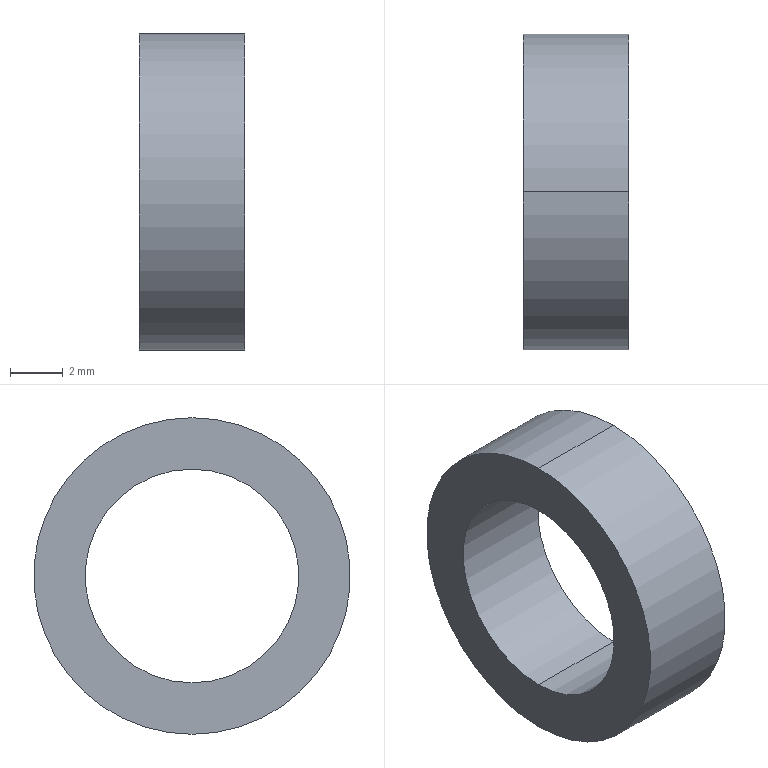Part | SolidWorks | features BaseBody 1 | 1 solid | 6 faces | box 4 x 12 x 12 mm | volume 246.269 mm3 | cylinder 4 | plane 2 | commonest cylinder face diameters 8.1 x2 12 x2
STEP:
#1=CARTESIAN_POINT('',(-2.,0.,-6.));
#2=VERTEX_POINT('',#1);
#3=CARTESIAN_POINT('',(-2.,0.,6.));
#4=VERTEX_POINT('',#3);
#5=CARTESIAN_POINT('',(-2.,0.,0.));
#6=DIRECTION('',(1.,0.,0.));
#7=DIRECTION('',(0.,0.,-1.));
#8=AXIS2_PLACEMENT_3D('',#5,#6,#7);
#9=CIRCLE('',#8,6.);
#10=EDGE_CURVE('',#2,#4,#9,.T.);
#11=ORIENTED_EDGE('',*,*,#10,.T.);
#12=CARTESIAN_POINT('',(2.,0.,6.));
#13=VERTEX_POINT('',#12);
#14=CARTESIAN_POINT('',(-2.,0.,6.));
#15=DIRECTION('',(1.,0.,0.));
#16=VECTOR('',#15,1000.);
#17=LINE('',#14,#16);
#18=EDGE_CURVE('',#4,#13,#17,.T.);
#19=ORIENTED_EDGE('',*,*,#18,.T.);
#20=CARTESIAN_POINT('',(2.,0.,-6.));
#21=VERTEX_POINT('',#20);
#22=CARTESIAN_POINT('',(2.,0.,0.));
#23=DIRECTION('',(-1.,0.,0.));
#24=DIRECTION('',(0.,0.,-1.));
#25=AXIS2_PLACEMENT_3D('',#22,#23,#24);
#26=CIRCLE('',#25,6.);
#27=EDGE_CURVE('',#13,#21,#26,.T.);
#28=ORIENTED_EDGE('',*,*,#27,.T.);
#29=CARTESIAN_POINT('',(-2.,0.,-6.));
#30=DIRECTION('',(1.,0.,0.));
#31=VECTOR('',#30,1000.);
#32=LINE('',#29,#31);
#33=EDGE_CURVE('',#2,#21,#32,.T.);
#34=ORIENTED_EDGE('',*,*,#33,.F.);
#35=EDGE_LOOP('',(#11,#19,#28,#34));
#36=FACE_OUTER_BOUND('',#35,.T.);
#37=CARTESIAN_POINT('',(-2.,0.,0.));
#38=DIRECTION('',(1.,0.,0.));
#39=DIRECTION('',(0.,0.,-1.));
#40=AXIS2_PLACEMENT_3D('',#37,#38,#39);
#41=CYLINDRICAL_SURFACE('',#40,6.);
#42=ADVANCED_FACE('',(#36),#41,.T.);
#43=CARTESIAN_POINT('',(-2.,0.,-4.05));
#44=VERTEX_POINT('',#43);
#45=CARTESIAN_POINT('',(-2.,0.,4.05));
#46=VERTEX_POINT('',#45);
#47=CARTESIAN_POINT('',(-2.,0.,0.));
#48=DIRECTION('',(-1.,0.,0.));
#49=DIRECTION('',(0.,0.,-1.));
#50=AXIS2_PLACEMENT_3D('',#47,#48,#49);
#51=CIRCLE('',#50,4.05);
#52=EDGE_CURVE('',#44,#46,#51,.T.);
#53=ORIENTED_EDGE('',*,*,#52,.T.);
#54=CARTESIAN_POINT('',(2.,0.,4.05));
#55=VERTEX_POINT('',#54);
#56=CARTESIAN_POINT('',(-3.,0.,4.05));
#57=DIRECTION('',(1.,0.,0.));
#58=VECTOR('',#57,1000.);
#59=LINE('',#56,#58);
#60=EDGE_CURVE('',#46,#55,#59,.T.);
#61=ORIENTED_EDGE('',*,*,#60,.T.);
#62=CARTESIAN_POINT('',(2.,0.,-4.05));
#63=VERTEX_POINT('',#62);
#64=CARTESIAN_POINT('',(2.,0.,0.));
#65=DIRECTION('',(-1.,0.,0.));
#66=DIRECTION('',(0.,0.,-1.));
#67=AXIS2_PLACEMENT_3D('',#64,#65,#66);
#68=CIRCLE('',#67,4.05);
#69=EDGE_CURVE('',#63,#55,#68,.T.);
#70=ORIENTED_EDGE('',*,*,#69,.F.);
#71=CARTESIAN_POINT('',(-3.,0.,-4.05));
#72=DIRECTION('',(1.,0.,0.));
#73=VECTOR('',#72,1000.);
#74=LINE('',#71,#73);
#75=EDGE_CURVE('',#44,#63,#74,.T.);
#76=ORIENTED_EDGE('',*,*,#75,.F.);
#77=EDGE_LOOP('',(#53,#61,#70,#76));
#78=FACE_OUTER_BOUND('',#77,.T.);
#79=CARTESIAN_POINT('',(-3.,0.,0.));
#80=DIRECTION('',(1.,0.,0.));
#81=DIRECTION('',(0.,0.,-1.));
#82=AXIS2_PLACEMENT_3D('',#79,#80,#81);
#83=CYLINDRICAL_SURFACE('',#82,4.05);
#84=ADVANCED_FACE('',(#78),#83,.F.);
#85=ORIENTED_EDGE('',*,*,#18,.F.);
#86=CARTESIAN_POINT('',(-2.,0.,0.));
#87=DIRECTION('',(1.,0.,0.));
#88=DIRECTION('',(0.,0.,-1.));
#89=AXIS2_PLACEMENT_3D('',#86,#87,#88);
#90=CIRCLE('',#89,6.);
#91=EDGE_CURVE('',#4,#2,#90,.T.);
#92=ORIENTED_EDGE('',*,*,#91,.T.);
#93=ORIENTED_EDGE('',*,*,#33,.T.);
#94=CARTESIAN_POINT('',(2.,0.,0.));
#95=DIRECTION('',(-1.,0.,0.));
#96=DIRECTION('',(0.,0.,-1.));
#97=AXIS2_PLACEMENT_3D('',#94,#95,#96);
#98=CIRCLE('',#97,6.);
#99=EDGE_CURVE('',#21,#13,#98,.T.);
#100=ORIENTED_EDGE('',*,*,#99,.T.);
#101=EDGE_LOOP('',(#85,#92,#93,#100));
#102=FACE_OUTER_BOUND('',#101,.T.);
#103=CARTESIAN_POINT('',(-2.,0.,0.));
#104=DIRECTION('',(1.,0.,0.));
#105=DIRECTION('',(0.,0.,-1.));
#106=AXIS2_PLACEMENT_3D('',#103,#104,#105);
#107=CYLINDRICAL_SURFACE('',#106,6.);
#108=ADVANCED_FACE('',(#102),#107,.T.);
#109=ORIENTED_EDGE('',*,*,#52,.F.);
#110=CARTESIAN_POINT('',(-2.,0.,0.));
#111=DIRECTION('',(-1.,0.,0.));
#112=DIRECTION('',(0.,0.,-1.));
#113=AXIS2_PLACEMENT_3D('',#110,#111,#112);
#114=CIRCLE('',#113,4.05);
#115=EDGE_CURVE('',#46,#44,#114,.T.);
#116=ORIENTED_EDGE('',*,*,#115,.F.);
#117=EDGE_LOOP('',(#109,#116));
#118=FACE_BOUND('',#117,.T.);
#119=ORIENTED_EDGE('',*,*,#10,.F.);
#120=ORIENTED_EDGE('',*,*,#91,.F.);
#121=EDGE_LOOP('',(#119,#120));
#122=FACE_OUTER_BOUND('',#121,.T.);
#123=CARTESIAN_POINT('',(-2.,0.,0.));
#124=DIRECTION('',(1.,0.,0.));
#125=DIRECTION('',(0.,0.,-1.));
#126=AXIS2_PLACEMENT_3D('',#123,#124,#125);
#127=PLANE('',#126);
#128=ADVANCED_FACE('',(#118,#122),#127,.F.);
#129=ORIENTED_EDGE('',*,*,#69,.T.);
#130=CARTESIAN_POINT('',(2.,0.,0.));
#131=DIRECTION('',(-1.,0.,0.));
#132=DIRECTION('',(0.,0.,-1.));
#133=AXIS2_PLACEMENT_3D('',#130,#131,#132);
#134=CIRCLE('',#133,4.05);
#135=EDGE_CURVE('',#55,#63,#134,.T.);
#136=ORIENTED_EDGE('',*,*,#135,.T.);
#137=EDGE_LOOP('',(#129,#136));
#138=FACE_BOUND('',#137,.T.);
#139=ORIENTED_EDGE('',*,*,#99,.F.);
#140=ORIENTED_EDGE('',*,*,#27,.F.);
#141=EDGE_LOOP('',(#139,#140));
#142=FACE_OUTER_BOUND('',#141,.T.);
#143=CARTESIAN_POINT('',(2.,0.,0.));
#144=DIRECTION('',(1.,0.,0.));
#145=DIRECTION('',(0.,0.,-1.));
#146=AXIS2_PLACEMENT_3D('',#143,#144,#145);
#147=PLANE('',#146);
#148=ADVANCED_FACE('',(#138,#142),#147,.T.);
#149=ORIENTED_EDGE('',*,*,#60,.F.);
#150=ORIENTED_EDGE('',*,*,#115,.T.);
#151=ORIENTED_EDGE('',*,*,#75,.T.);
#152=ORIENTED_EDGE('',*,*,#135,.F.);
#153=EDGE_LOOP('',(#149,#150,#151,#152));
#154=FACE_OUTER_BOUND('',#153,.T.);
#155=CARTESIAN_POINT('',(-3.,0.,0.));
#156=DIRECTION('',(1.,0.,0.));
#157=DIRECTION('',(0.,0.,-1.));
#158=AXIS2_PLACEMENT_3D('',#155,#156,#157);
#159=CYLINDRICAL_SURFACE('',#158,4.05);
#160=ADVANCED_FACE('',(#154),#159,.F.);
#161=CLOSED_SHELL('',(#42,#84,#108,#128,#148,#160));
#162=MANIFOLD_SOLID_BREP('',#161);
#163=CARTESIAN_POINT('',(0.,0.,0.));
#164=DIRECTION('',(0.,0.,1.));
#165=DIRECTION('',(1.,0.,0.));
#166=AXIS2_PLACEMENT_3D('',#163,#164,#165);
#167=(LENGTH_UNIT()NAMED_UNIT(*)SI_UNIT(.MILLI.,.METRE.));
#168=UNCERTAINTY_MEASURE_WITH_UNIT(LENGTH_MEASURE(0.00001),#167,'','');
#169=(NAMED_UNIT(*)PLANE_ANGLE_UNIT()SI_UNIT($,.RADIAN.));
#170=(NAMED_UNIT(*)SI_UNIT($,.STERADIAN.)SOLID_ANGLE_UNIT());
#171=(GEOMETRIC_REPRESENTATION_CONTEXT(3)GLOBAL_UNCERTAINTY_ASSIGNED_CONTEXT((#168))GLOBAL_UNIT_ASSIGNED_CONTEXT((#167,#169,#170))REPRESENTATION_CONTEXT('',''));
#172=ADVANCED_BREP_SHAPE_REPRESENTATION('',(#162,#166),#171);